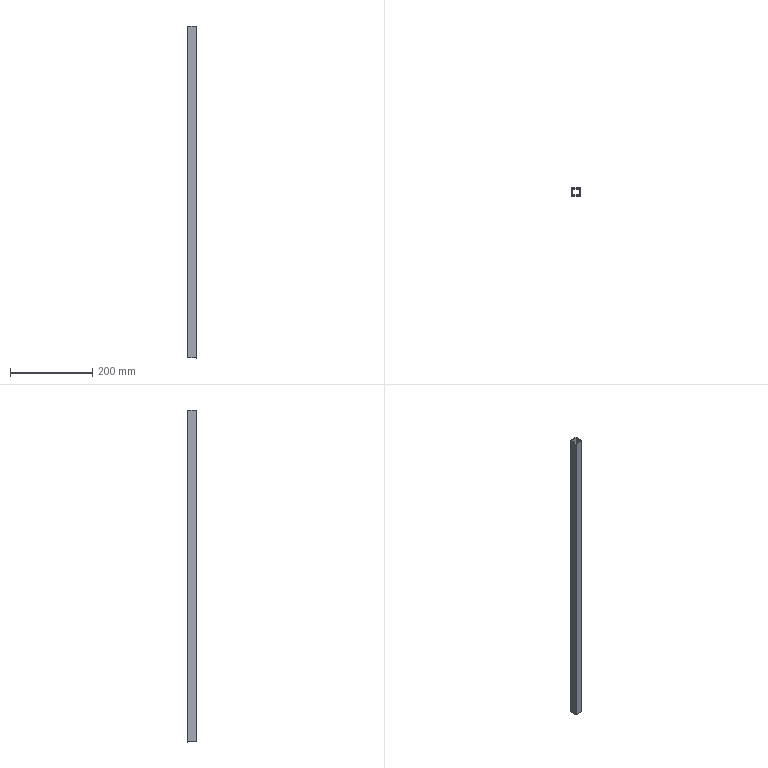Part | NX | features BREP 1 | 1 solid | 14 faces | box 20 x 20 x 807.958 mm | volume 116344 mm3 | plane 14
STEP:
#1=CARTESIAN_POINT('',(1628.587,678.,505.734));
#2=VERTEX_POINT('',#1);
#3=CARTESIAN_POINT('',(1628.587,678.,1313.692));
#4=VERTEX_POINT('',#3);
#5=CARTESIAN_POINT('',(1628.587,678.,909.713));
#6=DIRECTION('',(0.,0.,1.));
#7=VECTOR('',#6,1000.);
#8=LINE('',#5,#7);
#9=EDGE_CURVE('',#2,#4,#8,.T.);
#10=ORIENTED_EDGE('',*,*,#9,.T.);
#11=CARTESIAN_POINT('',(1608.587,678.,1313.692));
#12=VERTEX_POINT('',#11);
#13=CARTESIAN_POINT('',(1618.587,678.,1313.692));
#14=DIRECTION('',(1.,0.,0.));
#15=VECTOR('',#14,1000.);
#16=LINE('',#13,#15);
#17=EDGE_CURVE('',#12,#4,#16,.T.);
#18=ORIENTED_EDGE('',*,*,#17,.F.);
#19=CARTESIAN_POINT('',(1608.587,678.,505.763));
#20=VERTEX_POINT('',#19);
#21=CARTESIAN_POINT('',(1608.587,678.,505.763));
#22=CARTESIAN_POINT('',(1608.587,678.,667.348));
#23=CARTESIAN_POINT('',(1608.587,678.,828.934));
#24=CARTESIAN_POINT('',(1608.587,678.,990.52));
#25=CARTESIAN_POINT('',(1608.587,678.,1152.106));
#26=CARTESIAN_POINT('',(1608.587,678.,1313.692));
#27=B_SPLINE_CURVE_WITH_KNOTS('',5,(#21,#22,#23,#24,#25,#26),.UNSPECIFIED.,.F.,.F.,(6,6),(576.853,1384.783),.UNSPECIFIED.);
#28=EDGE_CURVE('',#20,#12,#27,.T.);
#29=ORIENTED_EDGE('',*,*,#28,.F.);
#30=CARTESIAN_POINT('',(1618.587,678.,505.748));
#31=DIRECTION('',(1.,0.,-0.001449));
#32=VECTOR('',#31,1000.);
#33=LINE('',#30,#32);
#34=EDGE_CURVE('',#20,#2,#33,.T.);
#35=ORIENTED_EDGE('',*,*,#34,.T.);
#36=EDGE_LOOP('',(#10,#18,#29,#35));
#37=FACE_BOUND('',#36,.T.);
#38=CARTESIAN_POINT('',(1628.587,678.,-71.091));
#39=DIRECTION('',(0.,-1.,0.));
#40=DIRECTION('',(0.,0.,1.));
#41=AXIS2_PLACEMENT_3D('',#38,#39,#40);
#42=PLANE('',#41);
#43=ADVANCED_FACE('',(#37),#42,.T.);
#44=CARTESIAN_POINT('',(1610.587,680.,505.76));
#45=VERTEX_POINT('',#44);
#46=CARTESIAN_POINT('',(1626.587,680.,505.737));
#47=VERTEX_POINT('',#46);
#48=CARTESIAN_POINT('',(1618.587,680.,505.748));
#49=DIRECTION('',(1.,0.,-0.001449));
#50=VECTOR('',#49,1000.);
#51=LINE('',#48,#50);
#52=EDGE_CURVE('',#45,#47,#51,.T.);
#53=ORIENTED_EDGE('',*,*,#52,.F.);
#54=CARTESIAN_POINT('',(1610.587,680.,1313.692));
#55=VERTEX_POINT('',#54);
#56=CARTESIAN_POINT('',(1610.587,680.,909.726));
#57=DIRECTION('',(0.,0.,1.));
#58=VECTOR('',#57,1000.);
#59=LINE('',#56,#58);
#60=EDGE_CURVE('',#45,#55,#59,.T.);
#61=ORIENTED_EDGE('',*,*,#60,.T.);
#62=CARTESIAN_POINT('',(1626.587,680.,1313.692));
#63=VERTEX_POINT('',#62);
#64=CARTESIAN_POINT('',(1618.587,680.,1313.692));
#65=DIRECTION('',(1.,0.,0.));
#66=VECTOR('',#65,1000.);
#67=LINE('',#64,#66);
#68=EDGE_CURVE('',#55,#63,#67,.T.);
#69=ORIENTED_EDGE('',*,*,#68,.T.);
#70=CARTESIAN_POINT('',(1626.587,680.,909.714));
#71=DIRECTION('',(0.,0.,1.));
#72=VECTOR('',#71,1000.);
#73=LINE('',#70,#72);
#74=EDGE_CURVE('',#47,#63,#73,.T.);
#75=ORIENTED_EDGE('',*,*,#74,.F.);
#76=EDGE_LOOP('',(#53,#61,#69,#75));
#77=FACE_BOUND('',#76,.T.);
#78=CARTESIAN_POINT('',(1628.587,680.,-71.091));
#79=DIRECTION('',(0.,-1.,0.));
#80=DIRECTION('',(0.,0.,1.));
#81=AXIS2_PLACEMENT_3D('',#78,#79,#80);
#82=PLANE('',#81);
#83=ADVANCED_FACE('',(#77),#82,.F.);
#84=ORIENTED_EDGE('',*,*,#28,.T.);
#85=CARTESIAN_POINT('',(1608.587,698.,1313.692));
#86=VERTEX_POINT('',#85);
#87=CARTESIAN_POINT('',(1608.587,688.,1313.692));
#88=DIRECTION('',(0.,1.,0.));
#89=VECTOR('',#88,1000.);
#90=LINE('',#87,#89);
#91=EDGE_CURVE('',#12,#86,#90,.T.);
#92=ORIENTED_EDGE('',*,*,#91,.T.);
#93=CARTESIAN_POINT('',(1608.587,698.,505.763));
#94=VERTEX_POINT('',#93);
#95=CARTESIAN_POINT('',(1608.587,698.,909.727));
#96=DIRECTION('',(0.,0.,1.));
#97=VECTOR('',#96,1000.);
#98=LINE('',#95,#97);
#99=EDGE_CURVE('',#94,#86,#98,.T.);
#100=ORIENTED_EDGE('',*,*,#99,.F.);
#101=CARTESIAN_POINT('',(1608.587,697.5,505.763));
#102=VERTEX_POINT('',#101);
#103=CARTESIAN_POINT('',(1608.587,697.5,505.763));
#104=CARTESIAN_POINT('',(1608.587,698.,505.763));
#105=B_SPLINE_CURVE_WITH_KNOTS('',1,(#103,#104),.UNSPECIFIED.,.F.,.F.,(2,2),(0.,0.4997),.UNSPECIFIED.);
#106=EDGE_CURVE('',#102,#94,#105,.T.);
#107=ORIENTED_EDGE('',*,*,#106,.F.);
#108=CARTESIAN_POINT('',(1608.587,687.75,505.763));
#109=DIRECTION('',(0.,1.,0.));
#110=VECTOR('',#109,1000.);
#111=LINE('',#108,#110);
#112=EDGE_CURVE('',#20,#102,#111,.T.);
#113=ORIENTED_EDGE('',*,*,#112,.F.);
#114=EDGE_LOOP('',(#84,#92,#100,#107,#113));
#115=FACE_BOUND('',#114,.T.);
#116=CARTESIAN_POINT('',(1608.587,688.,675.409));
#117=DIRECTION('',(-1.,0.,0.));
#118=DIRECTION('',(0.,0.,1.));
#119=AXIS2_PLACEMENT_3D('',#116,#117,#118);
#120=PLANE('',#119);
#121=ADVANCED_FACE('',(#115),#120,.T.);
#122=ORIENTED_EDGE('',*,*,#106,.T.);
#123=CARTESIAN_POINT('',(1628.587,698.,505.734));
#124=VERTEX_POINT('',#123);
#125=CARTESIAN_POINT('',(1618.587,698.,505.748));
#126=DIRECTION('',(1.,0.,-0.001449));
#127=VECTOR('',#126,1000.);
#128=LINE('',#125,#127);
#129=EDGE_CURVE('',#94,#124,#128,.T.);
#130=ORIENTED_EDGE('',*,*,#129,.T.);
#131=CARTESIAN_POINT('',(1628.587,697.5,505.734));
#132=VERTEX_POINT('',#131);
#133=CARTESIAN_POINT('',(1628.587,697.75,505.734));
#134=DIRECTION('',(0.,-1.,0.000000004));
#135=VECTOR('',#134,1000.);
#136=LINE('',#133,#135);
#137=EDGE_CURVE('',#124,#132,#136,.T.);
#138=ORIENTED_EDGE('',*,*,#137,.T.);
#139=CARTESIAN_POINT('',(1618.587,697.5,505.748));
#140=DIRECTION('',(1.,0.,-0.001449));
#141=VECTOR('',#140,1000.);
#142=LINE('',#139,#141);
#143=EDGE_CURVE('',#102,#132,#142,.T.);
#144=ORIENTED_EDGE('',*,*,#143,.F.);
#145=EDGE_LOOP('',(#122,#130,#138,#144));
#146=FACE_BOUND('',#145,.T.);
#147=CARTESIAN_POINT('',(1711.098,697.768,505.614));
#148=DIRECTION('',(0.001449,0.,1.));
#149=DIRECTION('',(1.,0.,-0.001449));
#150=AXIS2_PLACEMENT_3D('',#147,#148,#149);
#151=PLANE('',#150);
#152=ADVANCED_FACE('',(#146),#151,.F.);
#153=CARTESIAN_POINT('',(1628.587,698.,1313.692));
#154=VERTEX_POINT('',#153);
#155=CARTESIAN_POINT('',(1628.587,698.,909.713));
#156=DIRECTION('',(0.,0.,1.));
#157=VECTOR('',#156,1000.);
#158=LINE('',#155,#157);
#159=EDGE_CURVE('',#124,#154,#158,.T.);
#160=ORIENTED_EDGE('',*,*,#159,.T.);
#161=CARTESIAN_POINT('',(1628.587,688.,1313.692));
#162=DIRECTION('',(0.,-1.,0.));
#163=VECTOR('',#162,1000.);
#164=LINE('',#161,#163);
#165=EDGE_CURVE('',#154,#4,#164,.T.);
#166=ORIENTED_EDGE('',*,*,#165,.T.);
#167=ORIENTED_EDGE('',*,*,#9,.F.);
#168=CARTESIAN_POINT('',(1628.587,687.75,505.734));
#169=DIRECTION('',(0.,-1.,0.));
#170=VECTOR('',#169,1000.);
#171=LINE('',#168,#170);
#172=EDGE_CURVE('',#132,#2,#171,.T.);
#173=ORIENTED_EDGE('',*,*,#172,.F.);
#174=ORIENTED_EDGE('',*,*,#137,.F.);
#175=EDGE_LOOP('',(#160,#166,#167,#173,#174));
#176=FACE_BOUND('',#175,.T.);
#177=CARTESIAN_POINT('',(1628.587,698.,78.909));
#178=DIRECTION('',(1.,0.,0.));
#179=DIRECTION('',(0.,0.,1.));
#180=AXIS2_PLACEMENT_3D('',#177,#178,#179);
#181=PLANE('',#180);
#182=ADVANCED_FACE('',(#176),#181,.T.);
#183=CARTESIAN_POINT('',(1627.587,679.,1313.692));
#184=DIRECTION('',(-0.7071,0.7071,0.));
#185=VECTOR('',#184,1000.);
#186=LINE('',#183,#185);
#187=EDGE_CURVE('',#4,#63,#186,.T.);
#188=ORIENTED_EDGE('',*,*,#187,.T.);
#189=ORIENTED_EDGE('',*,*,#68,.F.);
#190=CARTESIAN_POINT('',(1609.587,679.,1313.692));
#191=DIRECTION('',(0.7071,0.7071,0.));
#192=VECTOR('',#191,1000.);
#193=LINE('',#190,#192);
#194=EDGE_CURVE('',#12,#55,#193,.T.);
#195=ORIENTED_EDGE('',*,*,#194,.F.);
#196=ORIENTED_EDGE('',*,*,#17,.T.);
#197=EDGE_LOOP('',(#188,#189,#195,#196));
#198=FACE_BOUND('',#197,.T.);
#199=CARTESIAN_POINT('',(1618.587,678.,1313.692));
#200=DIRECTION('',(0.,0.,-1.));
#201=DIRECTION('',(1.,0.,0.));
#202=AXIS2_PLACEMENT_3D('',#199,#200,#201);
#203=PLANE('',#202);
#204=ADVANCED_FACE('',(#198),#203,.F.);
#205=CARTESIAN_POINT('',(1610.587,696.,505.76));
#206=VERTEX_POINT('',#205);
#207=CARTESIAN_POINT('',(1610.587,688.,505.76));
#208=DIRECTION('',(0.,1.,0.));
#209=VECTOR('',#208,1000.);
#210=LINE('',#207,#209);
#211=EDGE_CURVE('',#45,#206,#210,.T.);
#212=ORIENTED_EDGE('',*,*,#211,.F.);
#213=ORIENTED_EDGE('',*,*,#52,.T.);
#214=CARTESIAN_POINT('',(1626.587,696.,505.737));
#215=VERTEX_POINT('',#214);
#216=CARTESIAN_POINT('',(1626.587,688.,505.737));
#217=DIRECTION('',(0.,-1.,0.));
#218=VECTOR('',#217,1000.);
#219=LINE('',#216,#218);
#220=EDGE_CURVE('',#215,#47,#219,.T.);
#221=ORIENTED_EDGE('',*,*,#220,.F.);
#222=CARTESIAN_POINT('',(1618.587,696.,505.748));
#223=DIRECTION('',(1.,0.,-0.001449));
#224=VECTOR('',#223,1000.);
#225=LINE('',#222,#224);
#226=EDGE_CURVE('',#206,#215,#225,.T.);
#227=ORIENTED_EDGE('',*,*,#226,.F.);
#228=EDGE_LOOP('',(#212,#213,#221,#227));
#229=FACE_BOUND('',#228,.T.);
#230=ORIENTED_EDGE('',*,*,#143,.T.);
#231=ORIENTED_EDGE('',*,*,#172,.T.);
#232=ORIENTED_EDGE('',*,*,#34,.F.);
#233=ORIENTED_EDGE('',*,*,#112,.T.);
#234=EDGE_LOOP('',(#230,#231,#232,#233));
#235=FACE_BOUND('',#234,.T.);
#236=CARTESIAN_POINT('',(1599.872,661.999,505.775));
#237=DIRECTION('',(-0.001449,0.,-1.));
#238=DIRECTION('',(1.,0.,-0.001449));
#239=AXIS2_PLACEMENT_3D('',#236,#237,#238);
#240=PLANE('',#239);
#241=ADVANCED_FACE('',(#229,#235),#240,.T.);
#242=ORIENTED_EDGE('',*,*,#211,.T.);
#243=CARTESIAN_POINT('',(1610.587,696.,1313.692));
#244=VERTEX_POINT('',#243);
#245=CARTESIAN_POINT('',(1610.587,696.,909.726));
#246=DIRECTION('',(0.,0.,1.));
#247=VECTOR('',#246,1000.);
#248=LINE('',#245,#247);
#249=EDGE_CURVE('',#206,#244,#248,.T.);
#250=ORIENTED_EDGE('',*,*,#249,.T.);
#251=CARTESIAN_POINT('',(1610.587,688.,1313.692));
#252=DIRECTION('',(0.,1.,0.));
#253=VECTOR('',#252,1000.);
#254=LINE('',#251,#253);
#255=EDGE_CURVE('',#55,#244,#254,.T.);
#256=ORIENTED_EDGE('',*,*,#255,.F.);
#257=ORIENTED_EDGE('',*,*,#60,.F.);
#258=EDGE_LOOP('',(#242,#250,#256,#257));
#259=FACE_BOUND('',#258,.T.);
#260=CARTESIAN_POINT('',(1610.587,680.,505.76));
#261=DIRECTION('',(-1.,0.,0.));
#262=DIRECTION('',(0.,0.,1.));
#263=AXIS2_PLACEMENT_3D('',#260,#261,#262);
#264=PLANE('',#263);
#265=ADVANCED_FACE('',(#259),#264,.F.);
#266=ORIENTED_EDGE('',*,*,#220,.T.);
#267=ORIENTED_EDGE('',*,*,#74,.T.);
#268=CARTESIAN_POINT('',(1626.587,696.,1313.692));
#269=VERTEX_POINT('',#268);
#270=CARTESIAN_POINT('',(1626.587,688.,1313.692));
#271=DIRECTION('',(0.,-1.,0.));
#272=VECTOR('',#271,1000.);
#273=LINE('',#270,#272);
#274=EDGE_CURVE('',#269,#63,#273,.T.);
#275=ORIENTED_EDGE('',*,*,#274,.F.);
#276=CARTESIAN_POINT('',(1626.587,696.,909.714));
#277=DIRECTION('',(0.,0.,1.));
#278=VECTOR('',#277,1000.);
#279=LINE('',#276,#278);
#280=EDGE_CURVE('',#215,#269,#279,.T.);
#281=ORIENTED_EDGE('',*,*,#280,.F.);
#282=EDGE_LOOP('',(#266,#267,#275,#281));
#283=FACE_BOUND('',#282,.T.);
#284=CARTESIAN_POINT('',(1626.587,698.,78.909));
#285=DIRECTION('',(1.,0.,0.));
#286=DIRECTION('',(0.,0.,1.));
#287=AXIS2_PLACEMENT_3D('',#284,#285,#286);
#288=PLANE('',#287);
#289=ADVANCED_FACE('',(#283),#288,.F.);
#290=CARTESIAN_POINT('',(1609.587,697.,1313.692));
#291=DIRECTION('',(0.7071,-0.7071,0.));
#292=VECTOR('',#291,1000.);
#293=LINE('',#290,#292);
#294=EDGE_CURVE('',#86,#244,#293,.T.);
#295=ORIENTED_EDGE('',*,*,#294,.F.);
#296=ORIENTED_EDGE('',*,*,#91,.F.);
#297=ORIENTED_EDGE('',*,*,#194,.T.);
#298=ORIENTED_EDGE('',*,*,#255,.T.);
#299=EDGE_LOOP('',(#295,#296,#297,#298));
#300=FACE_BOUND('',#299,.T.);
#301=CARTESIAN_POINT('',(1608.587,688.,1313.692));
#302=DIRECTION('',(0.,0.,1.));
#303=DIRECTION('',(1.,0.,0.));
#304=AXIS2_PLACEMENT_3D('',#301,#302,#303);
#305=PLANE('',#304);
#306=ADVANCED_FACE('',(#300),#305,.T.);
#307=ORIENTED_EDGE('',*,*,#129,.F.);
#308=ORIENTED_EDGE('',*,*,#99,.T.);
#309=CARTESIAN_POINT('',(1618.587,698.,1313.692));
#310=DIRECTION('',(1.,0.,0.));
#311=VECTOR('',#310,1000.);
#312=LINE('',#309,#311);
#313=EDGE_CURVE('',#86,#154,#312,.T.);
#314=ORIENTED_EDGE('',*,*,#313,.T.);
#315=ORIENTED_EDGE('',*,*,#159,.F.);
#316=EDGE_LOOP('',(#307,#308,#314,#315));
#317=FACE_BOUND('',#316,.T.);
#318=CARTESIAN_POINT('',(1628.587,698.,-71.091));
#319=DIRECTION('',(0.,-1.,0.));
#320=DIRECTION('',(0.,0.,1.));
#321=AXIS2_PLACEMENT_3D('',#318,#319,#320);
#322=PLANE('',#321);
#323=ADVANCED_FACE('',(#317),#322,.F.);
#324=ORIENTED_EDGE('',*,*,#187,.F.);
#325=ORIENTED_EDGE('',*,*,#165,.F.);
#326=CARTESIAN_POINT('',(1627.587,697.,1313.692));
#327=DIRECTION('',(-0.7071,-0.7071,0.));
#328=VECTOR('',#327,1000.);
#329=LINE('',#326,#328);
#330=EDGE_CURVE('',#154,#269,#329,.T.);
#331=ORIENTED_EDGE('',*,*,#330,.T.);
#332=ORIENTED_EDGE('',*,*,#274,.T.);
#333=EDGE_LOOP('',(#324,#325,#331,#332));
#334=FACE_BOUND('',#333,.T.);
#335=CARTESIAN_POINT('',(1628.587,688.,1313.692));
#336=DIRECTION('',(0.,0.,-1.));
#337=DIRECTION('',(1.,0.,0.));
#338=AXIS2_PLACEMENT_3D('',#335,#336,#337);
#339=PLANE('',#338);
#340=ADVANCED_FACE('',(#334),#339,.F.);
#341=ORIENTED_EDGE('',*,*,#280,.T.);
#342=CARTESIAN_POINT('',(1618.587,696.,1313.692));
#343=DIRECTION('',(1.,0.,0.));
#344=VECTOR('',#343,1000.);
#345=LINE('',#342,#344);
#346=EDGE_CURVE('',#244,#269,#345,.T.);
#347=ORIENTED_EDGE('',*,*,#346,.F.);
#348=ORIENTED_EDGE('',*,*,#249,.F.);
#349=ORIENTED_EDGE('',*,*,#226,.T.);
#350=EDGE_LOOP('',(#341,#347,#348,#349));
#351=FACE_BOUND('',#350,.T.);
#352=CARTESIAN_POINT('',(1628.587,696.,-71.091));
#353=DIRECTION('',(0.,-1.,0.));
#354=DIRECTION('',(0.,0.,1.));
#355=AXIS2_PLACEMENT_3D('',#352,#353,#354);
#356=PLANE('',#355);
#357=ADVANCED_FACE('',(#351),#356,.T.);
#358=ORIENTED_EDGE('',*,*,#346,.T.);
#359=ORIENTED_EDGE('',*,*,#330,.F.);
#360=ORIENTED_EDGE('',*,*,#313,.F.);
#361=ORIENTED_EDGE('',*,*,#294,.T.);
#362=EDGE_LOOP('',(#358,#359,#360,#361));
#363=FACE_BOUND('',#362,.T.);
#364=CARTESIAN_POINT('',(1618.587,698.,1313.692));
#365=DIRECTION('',(0.,0.,-1.));
#366=DIRECTION('',(1.,0.,0.));
#367=AXIS2_PLACEMENT_3D('',#364,#365,#366);
#368=PLANE('',#367);
#369=ADVANCED_FACE('',(#363),#368,.F.);
#370=CLOSED_SHELL('',(#43,#83,#121,#152,#182,#204,#241,#265,#289,#306,#323,#340,#357,#369));
#371=MANIFOLD_SOLID_BREP('',#370);
#372=(LENGTH_UNIT()NAMED_UNIT(*)SI_UNIT(.MILLI.,.METRE.));
#373=UNCERTAINTY_MEASURE_WITH_UNIT(LENGTH_MEASURE(0.00001),#372,'','');
#374=(NAMED_UNIT(*)PLANE_ANGLE_UNIT()SI_UNIT($,.RADIAN.));
#375=(NAMED_UNIT(*)SI_UNIT($,.STERADIAN.)SOLID_ANGLE_UNIT());
#376=(GEOMETRIC_REPRESENTATION_CONTEXT(3)GLOBAL_UNCERTAINTY_ASSIGNED_CONTEXT((#373))GLOBAL_UNIT_ASSIGNED_CONTEXT((#372,#374,#375))REPRESENTATION_CONTEXT('',''));
#377=ADVANCED_BREP_SHAPE_REPRESENTATION('',(#371),#376);